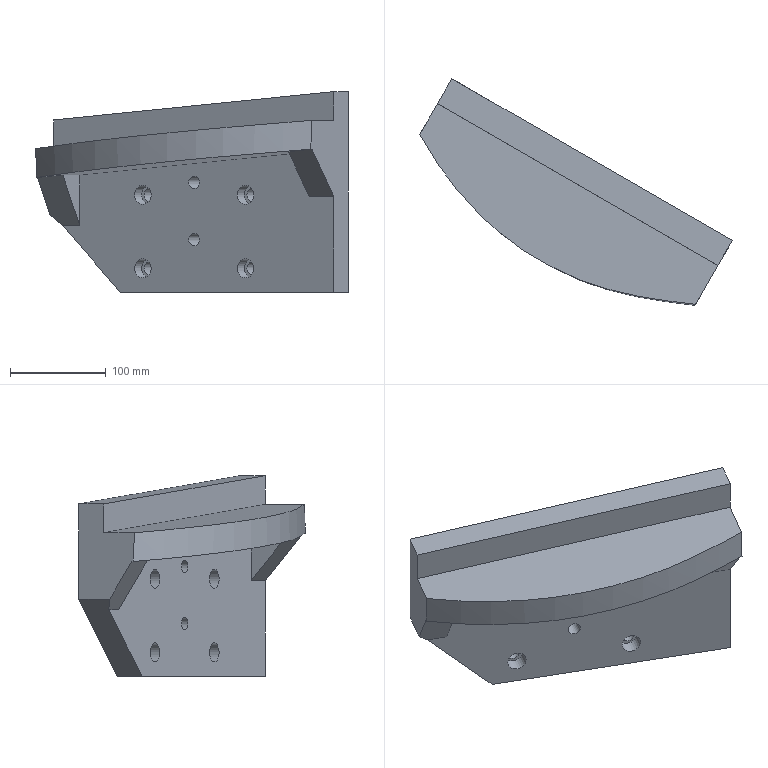Part | NX | features solid 2 | 1 solid | 29 faces | box 326.982 x 237.082 x 210.036 mm | volume 2654390 mm3 | plane 18 | cylinder 10 | spline 1 | commonest cylinder face diameters 14 x4 20 x4 13 x2
STEP:
#1=CARTESIAN_POINT('',(396.101,477.369,-114.823));
#2=VERTEX_POINT('',#1);
#3=CARTESIAN_POINT('',(683.197,297.298,-85.193));
#4=VERTEX_POINT('',#3);
#5=CARTESIAN_POINT('',(396.101,477.369,-114.823));
#6=CARTESIAN_POINT('',(397.889,474.16,-114.547));
#7=CARTESIAN_POINT('',(401.64,467.875,-113.988));
#8=CARTESIAN_POINT('',(407.329,458.495,-113.147));
#9=CARTESIAN_POINT('',(412.992,449.094,-112.307));
#10=CARTESIAN_POINT('',(421.058,436.951,-111.164));
#11=CARTESIAN_POINT('',(431.861,422.316,-109.705));
#12=CARTESIAN_POINT('',(445.96,405.613,-107.906));
#13=CARTESIAN_POINT('',(461.125,389.71,-106.062));
#14=CARTESIAN_POINT('',(477.463,374.718,-104.168));
#15=CARTESIAN_POINT('',(495.207,360.699,-102.21));
#16=CARTESIAN_POINT('',(510.706,350.446,-100.588));
#17=CARTESIAN_POINT('',(523.479,342.909,-99.29));
#18=CARTESIAN_POINT('',(533.18,337.485,-98.318));
#19=CARTESIAN_POINT('',(543.045,332.359,-97.346));
#20=CARTESIAN_POINT('',(556.498,326.084,-96.052));
#21=CARTESIAN_POINT('',(573.78,319.056,-94.436));
#22=CARTESIAN_POINT('',(602.455,309.974,-91.866));
#23=CARTESIAN_POINT('',(638.837,302.596,-88.786));
#24=CARTESIAN_POINT('',(668.432,299.158,-86.394));
#25=CARTESIAN_POINT('',(683.197,297.298,-85.193));
#26=B_SPLINE_CURVE_WITH_KNOTS('',3,(#5,#6,#7,#8,#9,#10,#11,#12,#13,#14,#15,#16,#17,#18,#19,#20,#21,#22,#23,#24,#25),.UNSPECIFIED.,.F.,.F.,(4,1,1,1,1,1,1,1,1,1,1,1,1,1,1,1,1,1,4),(0.6009,0.612,0.623,0.6341,0.6451,0.6673,0.6894,0.7115,0.7336,0.7557,0.7778,0.7889,0.7999,0.811,0.822,0.8441,0.8662,0.9105,0.9547),.UNSPECIFIED.);
#27=EDGE_CURVE('',#2,#4,#26,.T.);
#28=ORIENTED_EDGE('',*,*,#27,.F.);
#29=CARTESIAN_POINT('',(397.004,478.933,-114.823));
#30=VERTEX_POINT('',#29);
#31=CARTESIAN_POINT('',(514.016,681.604,-114.823));
#32=DIRECTION('',(-0.5,-0.866,0.));
#33=VECTOR('',#32,1000.);
#34=LINE('',#31,#33);
#35=EDGE_CURVE('',#30,#2,#34,.T.);
#36=ORIENTED_EDGE('',*,*,#35,.F.);
#37=CARTESIAN_POINT('',(423.492,461.475,-112.052));
#38=VERTEX_POINT('',#37);
#39=CARTESIAN_POINT('',(674.183,296.254,-85.831));
#40=DIRECTION('',(-0.8318,0.5482,-0.087));
#41=VECTOR('',#40,1000.);
#42=LINE('',#39,#41);
#43=EDGE_CURVE('',#30,#38,#42,.F.);
#44=ORIENTED_EDGE('',*,*,#43,.T.);
#45=CARTESIAN_POINT('',(441.442,492.565,-112.052));
#46=VERTEX_POINT('',#45);
#47=CARTESIAN_POINT('',(541.442,665.77,-112.052));
#48=DIRECTION('',(-0.5,-0.866,0.));
#49=VECTOR('',#48,1000.);
#50=LINE('',#47,#49);
#51=EDGE_CURVE('',#38,#46,#50,.F.);
#52=ORIENTED_EDGE('',*,*,#51,.T.);
#53=CARTESIAN_POINT('',(681.331,354.065,-87.818));
#54=VERTEX_POINT('',#53);
#55=CARTESIAN_POINT('',(713.906,335.258,-84.527));
#56=DIRECTION('',(-0.8627,0.4981,-0.08716));
#57=VECTOR('',#56,1000.);
#58=LINE('',#55,#57);
#59=EDGE_CURVE('',#46,#54,#58,.F.);
#60=ORIENTED_EDGE('',*,*,#59,.T.);
#61=CARTESIAN_POINT('',(659.681,316.566,-87.818));
#62=VERTEX_POINT('',#61);
#63=CARTESIAN_POINT('',(781.331,527.27,-87.818));
#64=DIRECTION('',(0.5,0.866,0.));
#65=VECTOR('',#64,1000.);
#66=LINE('',#63,#65);
#67=EDGE_CURVE('',#54,#62,#66,.F.);
#68=ORIENTED_EDGE('',*,*,#67,.T.);
#69=CARTESIAN_POINT('',(684.451,299.469,-85.193));
#70=VERTEX_POINT('',#69);
#71=CARTESIAN_POINT('',(674.552,306.302,-86.242));
#72=DIRECTION('',(-0.8199,0.5659,-0.08688));
#73=VECTOR('',#72,1000.);
#74=LINE('',#71,#73);
#75=EDGE_CURVE('',#62,#70,#74,.F.);
#76=ORIENTED_EDGE('',*,*,#75,.T.);
#77=CARTESIAN_POINT('',(694.536,316.937,-85.193));
#78=DIRECTION('',(-0.5,-0.866,0.));
#79=VECTOR('',#78,1000.);
#80=LINE('',#77,#79);
#81=EDGE_CURVE('',#70,#4,#80,.T.);
#82=ORIENTED_EDGE('',*,*,#81,.T.);
#83=EDGE_LOOP('',(#28,#36,#44,#52,#60,#68,#76,#82));
#84=FACE_BOUND('',#83,.T.);
#85=CARTESIAN_POINT('',(813.906,508.463,-84.527));
#86=DIRECTION('',(-0.07548,0.04358,0.9962));
#87=DIRECTION('',(0.9971,0.,0.07555));
#88=AXIS2_PLACEMENT_3D('',#85,#86,#87);
#89=PLANE('',#88);
#90=ADVANCED_FACE('',(#84),#89,.F.);
#91=CARTESIAN_POINT('',(606.133,397.481,-133.));
#92=VERTEX_POINT('',#91);
#93=CARTESIAN_POINT('',(614.793,392.481,-133.));
#94=DIRECTION('',(0.5,0.866,0.));
#95=DIRECTION('',(-0.866,0.5,0.));
#96=AXIS2_PLACEMENT_3D('',#93,#94,#95);
#97=CIRCLE('',#96,10.);
#98=EDGE_CURVE('',#92,#92,#97,.T.);
#99=ORIENTED_EDGE('',*,*,#98,.T.);
#100=EDGE_LOOP('',(#99));
#101=FACE_BOUND('',#100,.T.);
#102=CARTESIAN_POINT('',(498.745,459.481,-133.));
#103=VERTEX_POINT('',#102);
#104=CARTESIAN_POINT('',(507.406,454.481,-133.));
#105=DIRECTION('',(0.5,0.866,0.));
#106=DIRECTION('',(-0.866,0.5,0.));
#107=AXIS2_PLACEMENT_3D('',#104,#105,#106);
#108=CIRCLE('',#107,10.);
#109=EDGE_CURVE('',#103,#103,#108,.T.);
#110=ORIENTED_EDGE('',*,*,#109,.T.);
#111=EDGE_LOOP('',(#110));
#112=FACE_BOUND('',#111,.T.);
#113=CARTESIAN_POINT('',(606.133,397.481,-210.));
#114=VERTEX_POINT('',#113);
#115=CARTESIAN_POINT('',(614.793,392.481,-210.));
#116=DIRECTION('',(0.5,0.866,0.));
#117=DIRECTION('',(-0.866,0.5,0.));
#118=AXIS2_PLACEMENT_3D('',#115,#116,#117);
#119=CIRCLE('',#118,10.);
#120=EDGE_CURVE('',#114,#114,#119,.T.);
#121=ORIENTED_EDGE('',*,*,#120,.T.);
#122=EDGE_LOOP('',(#121));
#123=FACE_BOUND('',#122,.T.);
#124=CARTESIAN_POINT('',(498.745,459.481,-210.));
#125=VERTEX_POINT('',#124);
#126=CARTESIAN_POINT('',(507.406,454.481,-210.));
#127=DIRECTION('',(0.5,0.866,0.));
#128=DIRECTION('',(-0.866,0.5,0.));
#129=AXIS2_PLACEMENT_3D('',#126,#127,#128);
#130=CIRCLE('',#129,10.);
#131=EDGE_CURVE('',#125,#125,#130,.T.);
#132=ORIENTED_EDGE('',*,*,#131,.T.);
#133=EDGE_LOOP('',(#132));
#134=FACE_BOUND('',#133,.T.);
#135=CARTESIAN_POINT('',(555.47,426.731,-120.));
#136=VERTEX_POINT('',#135);
#137=CARTESIAN_POINT('',(561.099,423.481,-120.));
#138=DIRECTION('',(0.5,0.866,0.));
#139=DIRECTION('',(-0.866,0.5,0.));
#140=AXIS2_PLACEMENT_3D('',#137,#138,#139);
#141=CIRCLE('',#140,6.5);
#142=EDGE_CURVE('',#136,#136,#141,.T.);
#143=ORIENTED_EDGE('',*,*,#142,.T.);
#144=EDGE_LOOP('',(#143));
#145=FACE_BOUND('',#144,.T.);
#146=CARTESIAN_POINT('',(555.47,426.731,-180.));
#147=VERTEX_POINT('',#146);
#148=CARTESIAN_POINT('',(561.099,423.481,-180.));
#149=DIRECTION('',(0.5,0.866,0.));
#150=DIRECTION('',(-0.866,0.5,0.));
#151=AXIS2_PLACEMENT_3D('',#148,#149,#150);
#152=CIRCLE('',#151,6.5);
#153=EDGE_CURVE('',#147,#147,#152,.T.);
#154=ORIENTED_EDGE('',*,*,#153,.T.);
#155=EDGE_LOOP('',(#154));
#156=FACE_BOUND('',#155,.T.);
#157=CARTESIAN_POINT('',(423.478,502.937,-165.115));
#158=VERTEX_POINT('',#157);
#159=CARTESIAN_POINT('',(441.442,492.565,-165.115));
#160=VERTEX_POINT('',#159);
#161=CARTESIAN_POINT('',(721.314,330.981,-165.115));
#162=DIRECTION('',(0.866,-0.5,0.));
#163=VECTOR('',#162,1000.);
#164=LINE('',#161,#163);
#165=EDGE_CURVE('',#158,#160,#164,.T.);
#166=ORIENTED_EDGE('',*,*,#165,.F.);
#167=CARTESIAN_POINT('',(484.,467.994,-235.));
#168=VERTEX_POINT('',#167);
#169=CARTESIAN_POINT('',(477.876,471.529,-227.929));
#170=DIRECTION('',(0.6124,-0.3536,-0.7071));
#171=VECTOR('',#170,1000.);
#172=LINE('',#169,#171);
#173=EDGE_CURVE('',#158,#168,#172,.T.);
#174=ORIENTED_EDGE('',*,*,#173,.T.);
#175=CARTESIAN_POINT('',(707.312,339.065,-235.));
#176=VERTEX_POINT('',#175);
#177=CARTESIAN_POINT('',(561.099,423.481,-235.));
#178=DIRECTION('',(0.866,-0.5,0.));
#179=VECTOR('',#178,1000.);
#180=LINE('',#177,#179);
#181=EDGE_CURVE('',#168,#176,#180,.T.);
#182=ORIENTED_EDGE('',*,*,#181,.T.);
#183=CARTESIAN_POINT('',(707.312,339.065,-134.756));
#184=VERTEX_POINT('',#183);
#185=CARTESIAN_POINT('',(707.312,339.065,-45.974));
#186=DIRECTION('',(0.,0.,-1.));
#187=VECTOR('',#186,1000.);
#188=LINE('',#185,#187);
#189=EDGE_CURVE('',#176,#184,#188,.F.);
#190=ORIENTED_EDGE('',*,*,#189,.T.);
#191=CARTESIAN_POINT('',(681.331,354.065,-134.756));
#192=VERTEX_POINT('',#191);
#193=CARTESIAN_POINT('',(711.642,336.565,-134.756));
#194=DIRECTION('',(-0.866,0.5,0.));
#195=VECTOR('',#194,1000.);
#196=LINE('',#193,#195);
#197=EDGE_CURVE('',#184,#192,#196,.T.);
#198=ORIENTED_EDGE('',*,*,#197,.T.);
#199=CARTESIAN_POINT('',(681.331,354.065,-84.756));
#200=DIRECTION('',(0.,0.,1.));
#201=VECTOR('',#200,1000.);
#202=LINE('',#199,#201);
#203=EDGE_CURVE('',#54,#192,#202,.F.);
#204=ORIENTED_EDGE('',*,*,#203,.F.);
#205=ORIENTED_EDGE('',*,*,#59,.F.);
#206=CARTESIAN_POINT('',(441.442,492.565,-45.974));
#207=DIRECTION('',(0.,0.,1.));
#208=VECTOR('',#207,1000.);
#209=LINE('',#206,#208);
#210=EDGE_CURVE('',#160,#46,#209,.T.);
#211=ORIENTED_EDGE('',*,*,#210,.F.);
#212=EDGE_LOOP('',(#166,#174,#182,#190,#198,#204,#205,#211));
#213=FACE_BOUND('',#212,.T.);
#214=CARTESIAN_POINT('',(721.314,330.981,-45.974));
#215=DIRECTION('',(0.5,0.866,0.));
#216=DIRECTION('',(-0.866,0.5,0.));
#217=AXIS2_PLACEMENT_3D('',#214,#215,#216);
#218=PLANE('',#217);
#219=ADVANCED_FACE('',(#101,#112,#123,#134,#145,#156,#213),#218,.F.);
#220=CARTESIAN_POINT('',(395.33,476.033,-84.709));
#221=VERTEX_POINT('',#220);
#222=CARTESIAN_POINT('',(396.026,477.239,-111.933));
#223=VERTEX_POINT('',#222);
#224=CARTESIAN_POINT('',(395.33,476.033,-84.709));
#225=CARTESIAN_POINT('',(395.559,476.43,-93.784));
#226=CARTESIAN_POINT('',(395.791,476.832,-102.859));
#227=CARTESIAN_POINT('',(396.026,477.239,-111.933));
#228=B_SPLINE_CURVE_WITH_KNOTS('',3,(#224,#225,#226,#227),.UNSPECIFIED.,.F.,.F.,(4,4),(0.,0.02726),.UNSPECIFIED.);
#229=EDGE_CURVE('',#221,#223,#228,.T.);
#230=ORIENTED_EDGE('',*,*,#229,.T.);
#231=CARTESIAN_POINT('',(397.093,475.203,-110.115));
#232=VERTEX_POINT('',#231);
#233=CARTESIAN_POINT('',(397.093,475.203,-110.115));
#234=CARTESIAN_POINT('',(396.732,475.882,-110.718));
#235=CARTESIAN_POINT('',(396.377,476.561,-111.324));
#236=CARTESIAN_POINT('',(396.026,477.239,-111.933));
#237=B_SPLINE_CURVE_WITH_KNOTS('',3,(#233,#234,#235,#236),.UNSPECIFIED.,.F.,.F.,(4,4),(0.008928,0.01186),.UNSPECIFIED.);
#238=EDGE_CURVE('',#232,#223,#237,.T.);
#239=ORIENTED_EDGE('',*,*,#238,.F.);
#240=ORIENTED_EDGE('',*,*,#238,.T.);
#241=CARTESIAN_POINT('',(396.026,477.239,-111.933));
#242=CARTESIAN_POINT('',(396.051,477.283,-112.897));
#243=CARTESIAN_POINT('',(396.076,477.326,-113.86));
#244=CARTESIAN_POINT('',(396.101,477.369,-114.823));
#245=B_SPLINE_CURVE_WITH_KNOTS('',3,(#241,#242,#243,#244),.UNSPECIFIED.,.F.,.F.,(4,4),(0.,0.002894),.UNSPECIFIED.);
#246=EDGE_CURVE('',#223,#2,#245,.T.);
#247=ORIENTED_EDGE('',*,*,#246,.T.);
#248=ORIENTED_EDGE('',*,*,#27,.T.);
#249=CARTESIAN_POINT('',(683.747,298.251,-55.079));
#250=VERTEX_POINT('',#249);
#251=CARTESIAN_POINT('',(683.747,298.251,-55.079));
#252=CARTESIAN_POINT('',(683.564,297.933,-65.117));
#253=CARTESIAN_POINT('',(683.381,297.615,-75.155));
#254=CARTESIAN_POINT('',(683.197,297.298,-85.193));
#255=B_SPLINE_CURVE_WITH_KNOTS('',3,(#251,#252,#253,#254),.UNSPECIFIED.,.F.,.F.,(4,4),(0.188,0.2181),.UNSPECIFIED.);
#256=EDGE_CURVE('',#250,#4,#255,.T.);
#257=ORIENTED_EDGE('',*,*,#256,.F.);
#258=CARTESIAN_POINT('',(395.33,476.033,-84.709));
#259=CARTESIAN_POINT('',(397.169,472.823,-84.429));
#260=CARTESIAN_POINT('',(401.025,466.546,-83.862));
#261=CARTESIAN_POINT('',(406.683,457.029,-83.017));
#262=CARTESIAN_POINT('',(412.508,447.646,-82.165));
#263=CARTESIAN_POINT('',(420.747,435.51,-81.01));
#264=CARTESIAN_POINT('',(431.764,420.912,-79.537));
#265=CARTESIAN_POINT('',(446.092,404.273,-77.723));
#266=CARTESIAN_POINT('',(461.467,388.48,-75.868));
#267=CARTESIAN_POINT('',(478.064,373.608,-73.959));
#268=CARTESIAN_POINT('',(495.891,359.905,-72.009));
#269=CARTESIAN_POINT('',(511.426,349.911,-70.395));
#270=CARTESIAN_POINT('',(524.213,342.518,-69.103));
#271=CARTESIAN_POINT('',(537.147,335.392,-67.811));
#272=CARTESIAN_POINT('',(553.829,327.447,-66.2));
#273=CARTESIAN_POINT('',(574.692,319.23,-64.259));
#274=CARTESIAN_POINT('',(603.232,310.568,-61.718));
#275=CARTESIAN_POINT('',(632.26,304.87,-59.269));
#276=CARTESIAN_POINT('',(661.668,301.006,-56.872));
#277=CARTESIAN_POINT('',(676.389,299.178,-55.677));
#278=CARTESIAN_POINT('',(683.747,298.251,-55.079));
#279=B_SPLINE_CURVE_WITH_KNOTS('',3,(#258,#259,#260,#261,#262,#263,#264,#265,#266,#267,#268,#269,#270,#271,#272,#273,#274,#275,#276,#277,#278),.UNSPECIFIED.,.F.,.F.,(4,1,1,1,1,1,1,1,1,1,1,1,1,1,1,1,1,1,4),(1.587,1.598,1.609,1.62,1.631,1.654,1.676,1.698,1.721,1.743,1.765,1.776,1.788,1.81,1.832,1.855,1.899,1.921,1.944),.UNSPECIFIED.);
#280=EDGE_CURVE('',#221,#250,#279,.T.);
#281=ORIENTED_EDGE('',*,*,#280,.F.);
#282=EDGE_LOOP('',(#230,#239,#240,#247,#248,#257,#281));
#283=FACE_BOUND('',#282,.T.);
#284=CARTESIAN_POINT('',(395.055,479.257,-114.985));
#285=CARTESIAN_POINT('',(392.79,480.564,-85.099));
#286=CARTESIAN_POINT('',(396.892,475.94,-114.701));
#287=CARTESIAN_POINT('',(394.628,477.247,-84.815));
#288=CARTESIAN_POINT('',(400.689,469.378,-114.126));
#289=CARTESIAN_POINT('',(398.425,470.685,-84.24));
#290=CARTESIAN_POINT('',(406.636,459.688,-113.251));
#291=CARTESIAN_POINT('',(404.372,460.995,-83.366));
#292=CARTESIAN_POINT('',(412.461,449.918,-112.383));
#293=CARTESIAN_POINT('',(410.197,451.225,-82.497));
#294=CARTESIAN_POINT('',(420.799,437.301,-111.199));
#295=CARTESIAN_POINT('',(418.535,438.608,-81.313));
#296=CARTESIAN_POINT('',(431.995,422.116,-109.686));
#297=CARTESIAN_POINT('',(429.731,423.423,-79.801));
#298=CARTESIAN_POINT('',(446.695,404.772,-107.814));
#299=CARTESIAN_POINT('',(444.431,406.079,-77.928));
#300=CARTESIAN_POINT('',(462.398,388.446,-105.91));
#301=CARTESIAN_POINT('',(460.133,389.753,-76.024));
#302=CARTESIAN_POINT('',(479.215,373.225,-103.97));
#303=CARTESIAN_POINT('',(476.95,374.532,-74.084));
#304=CARTESIAN_POINT('',(497.155,359.295,-102.001));
#305=CARTESIAN_POINT('',(494.891,360.602,-72.116));
#306=CARTESIAN_POINT('',(512.973,349.034,-100.354));
#307=CARTESIAN_POINT('',(510.708,350.341,-70.468));
#308=CARTESIAN_POINT('',(526.067,341.44,-99.03));
#309=CARTESIAN_POINT('',(523.803,342.747,-69.144));
#310=CARTESIAN_POINT('',(539.307,334.131,-97.707));
#311=CARTESIAN_POINT('',(537.043,335.438,-67.821));
#312=CARTESIAN_POINT('',(556.33,326.026,-96.063));
#313=CARTESIAN_POINT('',(554.066,327.334,-66.177));
#314=CARTESIAN_POINT('',(577.514,317.721,-94.094));
#315=CARTESIAN_POINT('',(575.25,319.029,-64.208));
#316=CARTESIAN_POINT('',(606.314,309.057,-91.533));
#317=CARTESIAN_POINT('',(604.05,310.364,-61.647));
#318=CARTESIAN_POINT('',(635.776,303.349,-89.051));
#319=CARTESIAN_POINT('',(633.512,304.656,-59.165));
#320=CARTESIAN_POINT('',(665.66,299.492,-86.618));
#321=CARTESIAN_POINT('',(663.395,300.799,-56.732));
#322=CARTESIAN_POINT('',(680.653,297.618,-85.4));
#323=CARTESIAN_POINT('',(678.389,298.926,-55.514));
#324=CARTESIAN_POINT('',(688.143,296.675,-84.791));
#325=CARTESIAN_POINT('',(685.879,297.982,-54.906));
#326=B_SPLINE_SURFACE_WITH_KNOTS('',3,1,((#284,#285),(#286,#287),(#288,#289),(#290,#291),(#292,#293),(#294,#295),(#296,#297),(#298,#299),(#300,#301),(#302,#303),(#304,#305),(#306,#307),(#308,#309),(#310,#311),(#312,#313),(#314,#315),(#316,#317),(#318,#319),(#320,#321),(#322,#323),(#324,#325)),.SURF_OF_LINEAR_EXTRUSION.,.F.,.F.,.F.,(4,1,1,1,1,1,1,1,1,1,1,1,1,1,1,1,1,1,4),(2,2),(-0.003474,0.02642,0.05632,0.08622,0.1161,0.1759,0.2357,0.2955,0.3553,0.4151,0.4749,0.5048,0.5347,0.5945,0.6543,0.7141,0.8336,0.8934,0.9532),(0.,1.),.UNSPECIFIED.);
#327=ADVANCED_FACE('',(#283),#326,.T.);
#328=CARTESIAN_POINT('',(516.344,483.962,-133.));
#329=VERTEX_POINT('',#328);
#330=CARTESIAN_POINT('',(522.406,480.462,-133.));
#331=DIRECTION('',(0.5,0.866,0.));
#332=DIRECTION('',(-0.866,0.5,0.));
#333=AXIS2_PLACEMENT_3D('',#330,#331,#332);
#334=CIRCLE('',#333,7.);
#335=EDGE_CURVE('',#329,#329,#334,.F.);
#336=ORIENTED_EDGE('',*,*,#335,.T.);
#337=EDGE_LOOP('',(#336));
#338=FACE_BOUND('',#337,.T.);
#339=CARTESIAN_POINT('',(516.344,483.962,-210.));
#340=VERTEX_POINT('',#339);
#341=CARTESIAN_POINT('',(522.406,480.462,-210.));
#342=DIRECTION('',(0.5,0.866,0.));
#343=DIRECTION('',(-0.866,0.5,0.));
#344=AXIS2_PLACEMENT_3D('',#341,#342,#343);
#345=CIRCLE('',#344,7.);
#346=EDGE_CURVE('',#340,#340,#345,.F.);
#347=ORIENTED_EDGE('',*,*,#346,.T.);
#348=EDGE_LOOP('',(#347));
#349=FACE_BOUND('',#348,.T.);
#350=CARTESIAN_POINT('',(570.47,452.712,-180.));
#351=VERTEX_POINT('',#350);
#352=CARTESIAN_POINT('',(576.099,449.462,-180.));
#353=DIRECTION('',(0.5,0.866,0.));
#354=DIRECTION('',(-0.866,0.5,0.));
#355=AXIS2_PLACEMENT_3D('',#352,#353,#354);
#356=CIRCLE('',#355,6.5);
#357=EDGE_CURVE('',#351,#351,#356,.T.);
#358=ORIENTED_EDGE('',*,*,#357,.F.);
#359=EDGE_LOOP('',(#358));
#360=FACE_BOUND('',#359,.T.);
#361=CARTESIAN_POINT('',(623.731,421.962,-210.));
#362=VERTEX_POINT('',#361);
#363=CARTESIAN_POINT('',(629.793,418.462,-210.));
#364=DIRECTION('',(0.5,0.866,0.));
#365=DIRECTION('',(-0.866,0.5,0.));
#366=AXIS2_PLACEMENT_3D('',#363,#364,#365);
#367=CIRCLE('',#366,7.);
#368=EDGE_CURVE('',#362,#362,#367,.F.);
#369=ORIENTED_EDGE('',*,*,#368,.T.);
#370=EDGE_LOOP('',(#369));
#371=FACE_BOUND('',#370,.T.);
#372=CARTESIAN_POINT('',(570.47,452.712,-120.));
#373=VERTEX_POINT('',#372);
#374=CARTESIAN_POINT('',(576.099,449.462,-120.));
#375=DIRECTION('',(0.5,0.866,0.));
#376=DIRECTION('',(-0.866,0.5,0.));
#377=AXIS2_PLACEMENT_3D('',#374,#375,#376);
#378=CIRCLE('',#377,6.5);
#379=EDGE_CURVE('',#373,#373,#378,.T.);
#380=ORIENTED_EDGE('',*,*,#379,.F.);
#381=EDGE_LOOP('',(#380));
#382=FACE_BOUND('',#381,.T.);
#383=CARTESIAN_POINT('',(623.731,421.962,-133.));
#384=VERTEX_POINT('',#383);
#385=CARTESIAN_POINT('',(629.793,418.462,-133.));
#386=DIRECTION('',(0.5,0.866,0.));
#387=DIRECTION('',(-0.866,0.5,0.));
#388=AXIS2_PLACEMENT_3D('',#385,#386,#387);
#389=CIRCLE('',#388,7.);
#390=EDGE_CURVE('',#384,#384,#389,.F.);
#391=ORIENTED_EDGE('',*,*,#390,.T.);
#392=EDGE_LOOP('',(#391));
#393=FACE_BOUND('',#392,.T.);
#394=CARTESIAN_POINT('',(499.,493.975,-235.));
#395=VERTEX_POINT('',#394);
#396=CARTESIAN_POINT('',(722.312,365.046,-235.));
#397=VERTEX_POINT('',#396);
#398=CARTESIAN_POINT('',(736.314,356.962,-235.));
#399=DIRECTION('',(-0.866,0.5,0.));
#400=VECTOR('',#399,1000.);
#401=LINE('',#398,#400);
#402=EDGE_CURVE('',#395,#397,#401,.F.);
#403=ORIENTED_EDGE('',*,*,#402,.F.);
#404=CARTESIAN_POINT('',(429.016,534.38,-154.19));
#405=VERTEX_POINT('',#404);
#406=CARTESIAN_POINT('',(535.806,472.725,-277.5));
#407=DIRECTION('',(-0.6124,0.3536,0.7071));
#408=VECTOR('',#407,1000.);
#409=LINE('',#406,#408);
#410=EDGE_CURVE('',#395,#405,#409,.T.);
#411=ORIENTED_EDGE('',*,*,#410,.T.);
#412=CARTESIAN_POINT('',(429.016,534.38,-54.594));
#413=VERTEX_POINT('',#412);
#414=CARTESIAN_POINT('',(429.016,534.38,-45.974));
#415=DIRECTION('',(0.,0.,1.));
#416=VECTOR('',#415,1000.);
#417=LINE('',#414,#416);
#418=EDGE_CURVE('',#413,#405,#417,.F.);
#419=ORIENTED_EDGE('',*,*,#418,.F.);
#420=CARTESIAN_POINT('',(722.312,365.046,-24.964));
#421=VERTEX_POINT('',#420);
#422=CARTESIAN_POINT('',(574.771,450.228,-39.869));
#423=DIRECTION('',(-0.8627,0.4981,-0.08716));
#424=VECTOR('',#423,1000.);
#425=LINE('',#422,#424);
#426=EDGE_CURVE('',#413,#421,#425,.F.);
#427=ORIENTED_EDGE('',*,*,#426,.T.);
#428=CARTESIAN_POINT('',(722.312,365.046,-39.978));
#429=DIRECTION('',(0.,0.,1.));
#430=VECTOR('',#429,1000.);
#431=LINE('',#428,#430);
#432=EDGE_CURVE('',#421,#397,#431,.F.);
#433=ORIENTED_EDGE('',*,*,#432,.T.);
#434=EDGE_LOOP('',(#403,#411,#419,#427,#433));
#435=FACE_BOUND('',#434,.T.);
#436=CARTESIAN_POINT('',(736.314,356.962,-45.974));
#437=DIRECTION('',(0.5,0.866,0.));
#438=DIRECTION('',(-0.866,0.5,0.));
#439=AXIS2_PLACEMENT_3D('',#436,#437,#438);
#440=PLANE('',#439);
#441=ADVANCED_FACE('',(#338,#349,#360,#371,#382,#393,#435),#440,.T.);
#442=CARTESIAN_POINT('',(707.312,339.065,-24.964));
#443=VERTEX_POINT('',#442);
#444=CARTESIAN_POINT('',(707.312,339.065,-55.079));
#445=VERTEX_POINT('',#444);
#446=CARTESIAN_POINT('',(707.312,339.065,-39.978));
#447=DIRECTION('',(0.,0.,1.));
#448=VECTOR('',#447,1000.);
#449=LINE('',#446,#448);
#450=EDGE_CURVE('',#443,#445,#449,.F.);
#451=ORIENTED_EDGE('',*,*,#450,.F.);
#452=CARTESIAN_POINT('',(414.016,508.399,-54.594));
#453=VERTEX_POINT('',#452);
#454=CARTESIAN_POINT('',(559.771,424.248,-39.869));
#455=DIRECTION('',(-0.8627,0.4981,-0.08716));
#456=VECTOR('',#455,1000.);
#457=LINE('',#454,#456);
#458=EDGE_CURVE('',#453,#443,#457,.F.);
#459=ORIENTED_EDGE('',*,*,#458,.F.);
#460=CARTESIAN_POINT('',(414.016,508.399,-84.709));
#461=VERTEX_POINT('',#460);
#462=CARTESIAN_POINT('',(414.016,508.399,-45.974));
#463=DIRECTION('',(0.,0.,1.));
#464=VECTOR('',#463,1000.);
#465=LINE('',#462,#464);
#466=EDGE_CURVE('',#453,#461,#465,.F.);
#467=ORIENTED_EDGE('',*,*,#466,.T.);
#468=CARTESIAN_POINT('',(711.642,336.565,-54.641));
#469=DIRECTION('',(-0.8627,0.4981,-0.08716));
#470=VECTOR('',#469,1000.);
#471=LINE('',#468,#470);
#472=EDGE_CURVE('',#461,#445,#471,.F.);
#473=ORIENTED_EDGE('',*,*,#472,.T.);
#474=EDGE_LOOP('',(#451,#459,#467,#473));
#475=FACE_BOUND('',#474,.T.);
#476=CARTESIAN_POINT('',(721.314,330.981,-45.974));
#477=DIRECTION('',(0.5,0.866,0.));
#478=DIRECTION('',(-0.866,0.5,0.));
#479=AXIS2_PLACEMENT_3D('',#476,#477,#478);
#480=PLANE('',#479);
#481=ADVANCED_FACE('',(#475),#480,.F.);
#482=CARTESIAN_POINT('',(694.536,316.937,-24.964));
#483=DIRECTION('',(-0.5,-0.866,0.));
#484=VECTOR('',#483,1000.);
#485=LINE('',#482,#484);
#486=EDGE_CURVE('',#421,#443,#485,.T.);
#487=ORIENTED_EDGE('',*,*,#486,.F.);
#488=ORIENTED_EDGE('',*,*,#426,.F.);
#489=CARTESIAN_POINT('',(397.174,479.227,-54.594));
#490=DIRECTION('',(0.5,0.866,0.));
#491=VECTOR('',#490,1000.);
#492=LINE('',#489,#491);
#493=EDGE_CURVE('',#453,#413,#492,.T.);
#494=ORIENTED_EDGE('',*,*,#493,.F.);
#495=ORIENTED_EDGE('',*,*,#458,.T.);
#496=EDGE_LOOP('',(#487,#488,#494,#495));
#497=FACE_BOUND('',#496,.T.);
#498=CARTESIAN_POINT('',(612.271,515.18,-39.869));
#499=DIRECTION('',(-0.07548,0.04358,0.9962));
#500=DIRECTION('',(-0.5,-0.866,0.));
#501=AXIS2_PLACEMENT_3D('',#498,#499,#500);
#502=PLANE('',#501);
#503=ADVANCED_FACE('',(#497),#502,.T.);
#504=ORIENTED_EDGE('',*,*,#181,.F.);
#505=CARTESIAN_POINT('',(499.,493.975,-235.));
#506=DIRECTION('',(-0.5,-0.866,0.));
#507=VECTOR('',#506,1000.);
#508=LINE('',#505,#507);
#509=EDGE_CURVE('',#168,#395,#508,.F.);
#510=ORIENTED_EDGE('',*,*,#509,.T.);
#511=ORIENTED_EDGE('',*,*,#402,.T.);
#512=CARTESIAN_POINT('',(694.536,316.937,-235.));
#513=DIRECTION('',(0.5,0.866,0.));
#514=VECTOR('',#513,1000.);
#515=LINE('',#512,#514);
#516=EDGE_CURVE('',#176,#397,#515,.T.);
#517=ORIENTED_EDGE('',*,*,#516,.F.);
#518=EDGE_LOOP('',(#504,#510,#511,#517));
#519=FACE_BOUND('',#518,.T.);
#520=CARTESIAN_POINT('',(576.099,449.462,-235.));
#521=DIRECTION('',(0.,0.,-1.));
#522=DIRECTION('',(0.5,0.866,0.));
#523=AXIS2_PLACEMENT_3D('',#520,#521,#522);
#524=PLANE('',#523);
#525=ADVANCED_FACE('',(#519),#524,.T.);
#526=CARTESIAN_POINT('',(694.536,316.937,-55.079));
#527=DIRECTION('',(-0.5,-0.866,0.));
#528=VECTOR('',#527,1000.);
#529=LINE('',#526,#528);
#530=EDGE_CURVE('',#445,#250,#529,.T.);
#531=ORIENTED_EDGE('',*,*,#530,.F.);
#532=ORIENTED_EDGE('',*,*,#472,.F.);
#533=CARTESIAN_POINT('',(514.016,681.604,-84.709));
#534=DIRECTION('',(-0.5,-0.866,0.));
#535=VECTOR('',#534,1000.);
#536=LINE('',#533,#535);
#537=EDGE_CURVE('',#461,#221,#536,.T.);
#538=ORIENTED_EDGE('',*,*,#537,.T.);
#539=ORIENTED_EDGE('',*,*,#280,.T.);
#540=EDGE_LOOP('',(#531,#532,#538,#539));
#541=FACE_BOUND('',#540,.T.);
#542=CARTESIAN_POINT('',(811.642,509.77,-54.641));
#543=DIRECTION('',(-0.07548,0.04358,0.9962));
#544=DIRECTION('',(0.9971,0.,0.07555));
#545=AXIS2_PLACEMENT_3D('',#542,#543,#544);
#546=PLANE('',#545);
#547=ADVANCED_FACE('',(#541),#546,.T.);
#548=CARTESIAN_POINT('',(508.844,470.971,-210.));
#549=VERTEX_POINT('',#548);
#550=CARTESIAN_POINT('',(514.906,467.471,-210.));
#551=DIRECTION('',(0.5,0.866,0.));
#552=DIRECTION('',(-0.866,0.5,0.));
#553=AXIS2_PLACEMENT_3D('',#550,#551,#552);
#554=CIRCLE('',#553,7.);
#555=EDGE_CURVE('',#549,#549,#554,.T.);
#556=ORIENTED_EDGE('',*,*,#555,.F.);
#557=EDGE_LOOP('',(#556));
#558=FACE_BOUND('',#557,.T.);
#559=ORIENTED_EDGE('',*,*,#346,.F.);
#560=EDGE_LOOP('',(#559));
#561=FACE_BOUND('',#560,.T.);
#562=CARTESIAN_POINT('',(572.406,567.064,-210.));
#563=DIRECTION('',(-0.5,-0.866,0.));
#564=DIRECTION('',(0.,0.,-1.));
#565=AXIS2_PLACEMENT_3D('',#562,#563,#564);
#566=CYLINDRICAL_SURFACE('',#565,7.);
#567=ADVANCED_FACE('',(#558,#561),#566,.F.);
#568=ORIENTED_EDGE('',*,*,#357,.T.);
#569=EDGE_LOOP('',(#568));
#570=FACE_BOUND('',#569,.T.);
#571=ORIENTED_EDGE('',*,*,#153,.F.);
#572=EDGE_LOOP('',(#571));
#573=FACE_BOUND('',#572,.T.);
#574=CARTESIAN_POINT('',(626.099,536.064,-180.));
#575=DIRECTION('',(-0.5,-0.866,0.));
#576=DIRECTION('',(0.,0.,-1.));
#577=AXIS2_PLACEMENT_3D('',#574,#575,#576);
#578=CYLINDRICAL_SURFACE('',#577,6.5);
#579=ADVANCED_FACE('',(#570,#573),#578,.F.);
#580=CARTESIAN_POINT('',(616.231,408.971,-210.));
#581=VERTEX_POINT('',#580);
#582=CARTESIAN_POINT('',(622.293,405.471,-210.));
#583=DIRECTION('',(0.5,0.866,0.));
#584=DIRECTION('',(-0.866,0.5,0.));
#585=AXIS2_PLACEMENT_3D('',#582,#583,#584);
#586=CIRCLE('',#585,7.);
#587=EDGE_CURVE('',#581,#581,#586,.T.);
#588=ORIENTED_EDGE('',*,*,#587,.F.);
#589=EDGE_LOOP('',(#588));
#590=FACE_BOUND('',#589,.T.);
#591=ORIENTED_EDGE('',*,*,#368,.F.);
#592=EDGE_LOOP('',(#591));
#593=FACE_BOUND('',#592,.T.);
#594=CARTESIAN_POINT('',(679.793,505.064,-210.));
#595=DIRECTION('',(-0.5,-0.866,0.));
#596=DIRECTION('',(0.,0.,-1.));
#597=AXIS2_PLACEMENT_3D('',#594,#595,#596);
#598=CYLINDRICAL_SURFACE('',#597,7.);
#599=ADVANCED_FACE('',(#590,#593),#598,.F.);
#600=CARTESIAN_POINT('',(508.844,470.971,-133.));
#601=VERTEX_POINT('',#600);
#602=CARTESIAN_POINT('',(514.906,467.471,-133.));
#603=DIRECTION('',(0.5,0.866,0.));
#604=DIRECTION('',(-0.866,0.5,0.));
#605=AXIS2_PLACEMENT_3D('',#602,#603,#604);
#606=CIRCLE('',#605,7.);
#607=EDGE_CURVE('',#601,#601,#606,.T.);
#608=ORIENTED_EDGE('',*,*,#607,.F.);
#609=EDGE_LOOP('',(#608));
#610=FACE_BOUND('',#609,.T.);
#611=ORIENTED_EDGE('',*,*,#335,.F.);
#612=EDGE_LOOP('',(#611));
#613=FACE_BOUND('',#612,.T.);
#614=CARTESIAN_POINT('',(572.406,567.064,-133.));
#615=DIRECTION('',(-0.5,-0.866,0.));
#616=DIRECTION('',(0.,0.,-1.));
#617=AXIS2_PLACEMENT_3D('',#614,#615,#616);
#618=CYLINDRICAL_SURFACE('',#617,7.);
#619=ADVANCED_FACE('',(#610,#613),#618,.F.);
#620=ORIENTED_EDGE('',*,*,#379,.T.);
#621=EDGE_LOOP('',(#620));
#622=FACE_BOUND('',#621,.T.);
#623=ORIENTED_EDGE('',*,*,#142,.F.);
#624=EDGE_LOOP('',(#623));
#625=FACE_BOUND('',#624,.T.);
#626=CARTESIAN_POINT('',(626.099,536.064,-120.));
#627=DIRECTION('',(-0.5,-0.866,0.));
#628=DIRECTION('',(0.,0.,-1.));
#629=AXIS2_PLACEMENT_3D('',#626,#627,#628);
#630=CYLINDRICAL_SURFACE('',#629,6.5);
#631=ADVANCED_FACE('',(#622,#625),#630,.F.);
#632=CARTESIAN_POINT('',(616.231,408.971,-133.));
#633=VERTEX_POINT('',#632);
#634=CARTESIAN_POINT('',(622.293,405.471,-133.));
#635=DIRECTION('',(0.5,0.866,0.));
#636=DIRECTION('',(-0.866,0.5,0.));
#637=AXIS2_PLACEMENT_3D('',#634,#635,#636);
#638=CIRCLE('',#637,7.);
#639=EDGE_CURVE('',#633,#633,#638,.T.);
#640=ORIENTED_EDGE('',*,*,#639,.F.);
#641=EDGE_LOOP('',(#640));
#642=FACE_BOUND('',#641,.T.);
#643=ORIENTED_EDGE('',*,*,#390,.F.);
#644=EDGE_LOOP('',(#643));
#645=FACE_BOUND('',#644,.T.);
#646=CARTESIAN_POINT('',(679.793,505.064,-133.));
#647=DIRECTION('',(-0.5,-0.866,0.));
#648=DIRECTION('',(0.,0.,-1.));
#649=AXIS2_PLACEMENT_3D('',#646,#647,#648);
#650=CYLINDRICAL_SURFACE('',#649,7.);
#651=ADVANCED_FACE('',(#642,#645),#650,.F.);
#652=ORIENTED_EDGE('',*,*,#418,.T.);
#653=CARTESIAN_POINT('',(410.321,501.998,-154.19));
#654=VERTEX_POINT('',#653);
#655=CARTESIAN_POINT('',(429.016,534.38,-154.19));
#656=DIRECTION('',(0.5,0.866,0.));
#657=VECTOR('',#656,1000.);
#658=LINE('',#655,#657);
#659=EDGE_CURVE('',#405,#654,#658,.F.);
#660=ORIENTED_EDGE('',*,*,#659,.T.);
#661=CARTESIAN_POINT('',(397.103,479.103,-115.115));
#662=DIRECTION('',(-0.2802,-0.4853,0.8283));
#663=VECTOR('',#662,1000.);
#664=LINE('',#661,#663);
#665=EDGE_CURVE('',#30,#654,#664,.F.);
#666=ORIENTED_EDGE('',*,*,#665,.F.);
#667=ORIENTED_EDGE('',*,*,#35,.T.);
#668=ORIENTED_EDGE('',*,*,#246,.F.);
#669=ORIENTED_EDGE('',*,*,#229,.F.);
#670=ORIENTED_EDGE('',*,*,#537,.F.);
#671=ORIENTED_EDGE('',*,*,#466,.F.);
#672=ORIENTED_EDGE('',*,*,#493,.T.);
#673=EDGE_LOOP('',(#652,#660,#666,#667,#668,#669,#670,#671,#672));
#674=FACE_BOUND('',#673,.T.);
#675=CARTESIAN_POINT('',(397.174,479.227,-70.199));
#676=DIRECTION('',(-0.866,0.5,0.));
#677=DIRECTION('',(-0.5,-0.866,0.));
#678=AXIS2_PLACEMENT_3D('',#675,#676,#677);
#679=PLANE('',#678);
#680=ADVANCED_FACE('',(#674),#679,.T.);
#681=ORIENTED_EDGE('',*,*,#256,.T.);
#682=ORIENTED_EDGE('',*,*,#81,.F.);
#683=CARTESIAN_POINT('',(684.249,299.12,-84.756));
#684=DIRECTION('',(0.339,0.5872,-0.735));
#685=VECTOR('',#684,1000.);
#686=LINE('',#683,#685);
#687=EDGE_CURVE('',#184,#70,#686,.F.);
#688=ORIENTED_EDGE('',*,*,#687,.F.);
#689=ORIENTED_EDGE('',*,*,#189,.F.);
#690=ORIENTED_EDGE('',*,*,#516,.T.);
#691=ORIENTED_EDGE('',*,*,#432,.F.);
#692=ORIENTED_EDGE('',*,*,#486,.T.);
#693=ORIENTED_EDGE('',*,*,#450,.T.);
#694=ORIENTED_EDGE('',*,*,#530,.T.);
#695=EDGE_LOOP('',(#681,#682,#688,#689,#690,#691,#692,#693,#694));
#696=FACE_BOUND('',#695,.T.);
#697=CARTESIAN_POINT('',(694.536,316.937,-39.978));
#698=DIRECTION('',(0.866,-0.5,0.));
#699=DIRECTION('',(0.5,0.866,0.));
#700=AXIS2_PLACEMENT_3D('',#697,#698,#699);
#701=PLANE('',#700);
#702=ADVANCED_FACE('',(#696),#701,.T.);
#703=CARTESIAN_POINT('',(506.245,472.471,-210.));
#704=VERTEX_POINT('',#703);
#705=CARTESIAN_POINT('',(514.906,467.471,-210.));
#706=DIRECTION('',(0.5,0.866,0.));
#707=DIRECTION('',(-0.866,0.5,0.));
#708=AXIS2_PLACEMENT_3D('',#705,#706,#707);
#709=CIRCLE('',#708,10.);
#710=EDGE_CURVE('',#704,#704,#709,.T.);
#711=ORIENTED_EDGE('',*,*,#710,.T.);
#712=EDGE_LOOP('',(#711));
#713=FACE_BOUND('',#712,.T.);
#714=ORIENTED_EDGE('',*,*,#131,.F.);
#715=EDGE_LOOP('',(#714));
#716=FACE_BOUND('',#715,.T.);
#717=CARTESIAN_POINT('',(507.406,454.481,-210.));
#718=DIRECTION('',(0.5,0.866,0.));
#719=DIRECTION('',(-0.866,0.5,0.));
#720=AXIS2_PLACEMENT_3D('',#717,#718,#719);
#721=CYLINDRICAL_SURFACE('',#720,10.);
#722=ADVANCED_FACE('',(#713,#716),#721,.F.);
#723=ORIENTED_EDGE('',*,*,#710,.F.);
#724=EDGE_LOOP('',(#723));
#725=FACE_BOUND('',#724,.T.);
#726=ORIENTED_EDGE('',*,*,#555,.T.);
#727=EDGE_LOOP('',(#726));
#728=FACE_BOUND('',#727,.T.);
#729=CARTESIAN_POINT('',(514.906,467.471,-210.));
#730=DIRECTION('',(-0.5,-0.866,0.));
#731=DIRECTION('',(0.866,-0.5,0.));
#732=AXIS2_PLACEMENT_3D('',#729,#730,#731);
#733=PLANE('',#732);
#734=ADVANCED_FACE('',(#725,#728),#733,.T.);
#735=CARTESIAN_POINT('',(613.633,410.471,-210.));
#736=VERTEX_POINT('',#735);
#737=CARTESIAN_POINT('',(622.293,405.471,-210.));
#738=DIRECTION('',(0.5,0.866,0.));
#739=DIRECTION('',(-0.866,0.5,0.));
#740=AXIS2_PLACEMENT_3D('',#737,#738,#739);
#741=CIRCLE('',#740,10.);
#742=EDGE_CURVE('',#736,#736,#741,.T.);
#743=ORIENTED_EDGE('',*,*,#742,.T.);
#744=EDGE_LOOP('',(#743));
#745=FACE_BOUND('',#744,.T.);
#746=ORIENTED_EDGE('',*,*,#120,.F.);
#747=EDGE_LOOP('',(#746));
#748=FACE_BOUND('',#747,.T.);
#749=CARTESIAN_POINT('',(614.793,392.481,-210.));
#750=DIRECTION('',(0.5,0.866,0.));
#751=DIRECTION('',(-0.866,0.5,0.));
#752=AXIS2_PLACEMENT_3D('',#749,#750,#751);
#753=CYLINDRICAL_SURFACE('',#752,10.);
#754=ADVANCED_FACE('',(#745,#748),#753,.F.);
#755=ORIENTED_EDGE('',*,*,#742,.F.);
#756=EDGE_LOOP('',(#755));
#757=FACE_BOUND('',#756,.T.);
#758=ORIENTED_EDGE('',*,*,#587,.T.);
#759=EDGE_LOOP('',(#758));
#760=FACE_BOUND('',#759,.T.);
#761=CARTESIAN_POINT('',(622.293,405.471,-210.));
#762=DIRECTION('',(-0.5,-0.866,0.));
#763=DIRECTION('',(0.866,-0.5,0.));
#764=AXIS2_PLACEMENT_3D('',#761,#762,#763);
#765=PLANE('',#764);
#766=ADVANCED_FACE('',(#757,#760),#765,.T.);
#767=CARTESIAN_POINT('',(506.245,472.471,-133.));
#768=VERTEX_POINT('',#767);
#769=CARTESIAN_POINT('',(514.906,467.471,-133.));
#770=DIRECTION('',(0.5,0.866,0.));
#771=DIRECTION('',(-0.866,0.5,0.));
#772=AXIS2_PLACEMENT_3D('',#769,#770,#771);
#773=CIRCLE('',#772,10.);
#774=EDGE_CURVE('',#768,#768,#773,.T.);
#775=ORIENTED_EDGE('',*,*,#774,.T.);
#776=EDGE_LOOP('',(#775));
#777=FACE_BOUND('',#776,.T.);
#778=ORIENTED_EDGE('',*,*,#109,.F.);
#779=EDGE_LOOP('',(#778));
#780=FACE_BOUND('',#779,.T.);
#781=CARTESIAN_POINT('',(507.406,454.481,-133.));
#782=DIRECTION('',(0.5,0.866,0.));
#783=DIRECTION('',(-0.866,0.5,0.));
#784=AXIS2_PLACEMENT_3D('',#781,#782,#783);
#785=CYLINDRICAL_SURFACE('',#784,10.);
#786=ADVANCED_FACE('',(#777,#780),#785,.F.);
#787=ORIENTED_EDGE('',*,*,#774,.F.);
#788=EDGE_LOOP('',(#787));
#789=FACE_BOUND('',#788,.T.);
#790=ORIENTED_EDGE('',*,*,#607,.T.);
#791=EDGE_LOOP('',(#790));
#792=FACE_BOUND('',#791,.T.);
#793=CARTESIAN_POINT('',(514.906,467.471,-133.));
#794=DIRECTION('',(-0.5,-0.866,0.));
#795=DIRECTION('',(0.866,-0.5,0.));
#796=AXIS2_PLACEMENT_3D('',#793,#794,#795);
#797=PLANE('',#796);
#798=ADVANCED_FACE('',(#789,#792),#797,.T.);
#799=CARTESIAN_POINT('',(613.633,410.471,-133.));
#800=VERTEX_POINT('',#799);
#801=CARTESIAN_POINT('',(622.293,405.471,-133.));
#802=DIRECTION('',(0.5,0.866,0.));
#803=DIRECTION('',(-0.866,0.5,0.));
#804=AXIS2_PLACEMENT_3D('',#801,#802,#803);
#805=CIRCLE('',#804,10.);
#806=EDGE_CURVE('',#800,#800,#805,.T.);
#807=ORIENTED_EDGE('',*,*,#806,.T.);
#808=EDGE_LOOP('',(#807));
#809=FACE_BOUND('',#808,.T.);
#810=ORIENTED_EDGE('',*,*,#98,.F.);
#811=EDGE_LOOP('',(#810));
#812=FACE_BOUND('',#811,.T.);
#813=CARTESIAN_POINT('',(614.793,392.481,-133.));
#814=DIRECTION('',(0.5,0.866,0.));
#815=DIRECTION('',(-0.866,0.5,0.));
#816=AXIS2_PLACEMENT_3D('',#813,#814,#815);
#817=CYLINDRICAL_SURFACE('',#816,10.);
#818=ADVANCED_FACE('',(#809,#812),#817,.F.);
#819=ORIENTED_EDGE('',*,*,#806,.F.);
#820=EDGE_LOOP('',(#819));
#821=FACE_BOUND('',#820,.T.);
#822=ORIENTED_EDGE('',*,*,#639,.T.);
#823=EDGE_LOOP('',(#822));
#824=FACE_BOUND('',#823,.T.);
#825=CARTESIAN_POINT('',(622.293,405.471,-133.));
#826=DIRECTION('',(-0.5,-0.866,0.));
#827=DIRECTION('',(0.866,-0.5,0.));
#828=AXIS2_PLACEMENT_3D('',#825,#826,#827);
#829=PLANE('',#828);
#830=ADVANCED_FACE('',(#821,#824),#829,.T.);
#831=ORIENTED_EDGE('',*,*,#75,.F.);
#832=CARTESIAN_POINT('',(668.871,332.485,-107.744));
#833=DIRECTION('',(-0.339,-0.5872,0.735));
#834=VECTOR('',#833,1000.);
#835=LINE('',#832,#834);
#836=EDGE_CURVE('',#192,#62,#835,.T.);
#837=ORIENTED_EDGE('',*,*,#836,.F.);
#838=ORIENTED_EDGE('',*,*,#197,.F.);
#839=ORIENTED_EDGE('',*,*,#687,.T.);
#840=EDGE_LOOP('',(#831,#837,#838,#839));
#841=FACE_BOUND('',#840,.T.);
#842=CARTESIAN_POINT('',(688.579,296.62,-84.756));
#843=DIRECTION('',(0.3675,0.6365,0.678));
#844=DIRECTION('',(0.,-0.7291,0.6844));
#845=AXIS2_PLACEMENT_3D('',#842,#843,#844);
#846=PLANE('',#845);
#847=ADVANCED_FACE('',(#841),#846,.F.);
#848=ORIENTED_EDGE('',*,*,#67,.F.);
#849=ORIENTED_EDGE('',*,*,#203,.T.);
#850=ORIENTED_EDGE('',*,*,#836,.T.);
#851=EDGE_LOOP('',(#848,#849,#850));
#852=FACE_BOUND('',#851,.T.);
#853=CARTESIAN_POINT('',(681.331,354.065,-84.756));
#854=DIRECTION('',(0.866,-0.5,0.));
#855=DIRECTION('',(0.5,0.866,0.));
#856=AXIS2_PLACEMENT_3D('',#853,#854,#855);
#857=PLANE('',#856);
#858=ADVANCED_FACE('',(#852),#857,.F.);
#859=ORIENTED_EDGE('',*,*,#665,.T.);
#860=CARTESIAN_POINT('',(494.982,508.038,-224.489));
#861=DIRECTION('',(0.7682,0.0548,-0.6379));
#862=VECTOR('',#861,1000.);
#863=LINE('',#860,#862);
#864=EDGE_CURVE('',#654,#158,#863,.T.);
#865=ORIENTED_EDGE('',*,*,#864,.T.);
#866=ORIENTED_EDGE('',*,*,#165,.T.);
#867=CARTESIAN_POINT('',(424.528,463.269,-115.115));
#868=DIRECTION('',(0.2802,0.4853,-0.8283));
#869=VECTOR('',#868,1000.);
#870=LINE('',#867,#869);
#871=EDGE_CURVE('',#38,#160,#870,.T.);
#872=ORIENTED_EDGE('',*,*,#871,.F.);
#873=ORIENTED_EDGE('',*,*,#43,.F.);
#874=EDGE_LOOP('',(#859,#865,#866,#872,#873));
#875=FACE_BOUND('',#874,.T.);
#876=CARTESIAN_POINT('',(394.217,480.769,-115.115));
#877=DIRECTION('',(0.4141,0.7173,0.5604));
#878=DIRECTION('',(0.,-0.6156,0.788));
#879=AXIS2_PLACEMENT_3D('',#876,#877,#878);
#880=PLANE('',#879);
#881=ADVANCED_FACE('',(#875),#880,.F.);
#882=ORIENTED_EDGE('',*,*,#51,.F.);
#883=ORIENTED_EDGE('',*,*,#871,.T.);
#884=ORIENTED_EDGE('',*,*,#210,.T.);
#885=EDGE_LOOP('',(#882,#883,#884));
#886=FACE_BOUND('',#885,.T.);
#887=CARTESIAN_POINT('',(424.528,463.269,-115.115));
#888=DIRECTION('',(-0.866,0.5,0.));
#889=DIRECTION('',(-0.5,-0.866,0.));
#890=AXIS2_PLACEMENT_3D('',#887,#888,#889);
#891=PLANE('',#890);
#892=ADVANCED_FACE('',(#886),#891,.F.);
#893=ORIENTED_EDGE('',*,*,#864,.F.);
#894=ORIENTED_EDGE('',*,*,#659,.F.);
#895=ORIENTED_EDGE('',*,*,#410,.F.);
#896=ORIENTED_EDGE('',*,*,#509,.F.);
#897=ORIENTED_EDGE('',*,*,#173,.F.);
#898=EDGE_LOOP('',(#893,#894,#895,#896,#897));
#899=FACE_BOUND('',#898,.T.);
#900=CARTESIAN_POINT('',(492.876,497.51,-227.929));
#901=DIRECTION('',(-0.6124,0.3536,-0.7071));
#902=DIRECTION('',(-0.7559,0.,0.6547));
#903=AXIS2_PLACEMENT_3D('',#900,#901,#902);
#904=PLANE('',#903);
#905=ADVANCED_FACE('',(#899),#904,.T.);
#906=CLOSED_SHELL('',(#90,#219,#327,#441,#481,#503,#525,#547,#567,#579,#599,#619,#631,#651,#680,#702,#722,#734,#754,#766,#786,#798,#818,#830,#847,#858,#881,#892,#905));
#907=MANIFOLD_SOLID_BREP('',#906);
#908=(LENGTH_UNIT()NAMED_UNIT(*)SI_UNIT(.MILLI.,.METRE.));
#909=UNCERTAINTY_MEASURE_WITH_UNIT(LENGTH_MEASURE(0.0508),#908,'','');
#910=(NAMED_UNIT(*)PLANE_ANGLE_UNIT()SI_UNIT($,.RADIAN.));
#911=(NAMED_UNIT(*)SI_UNIT($,.STERADIAN.)SOLID_ANGLE_UNIT());
#912=(GEOMETRIC_REPRESENTATION_CONTEXT(3)GLOBAL_UNCERTAINTY_ASSIGNED_CONTEXT((#909))GLOBAL_UNIT_ASSIGNED_CONTEXT((#908,#910,#911))REPRESENTATION_CONTEXT('',''));
#913=ADVANCED_BREP_SHAPE_REPRESENTATION('',(#907),#912);